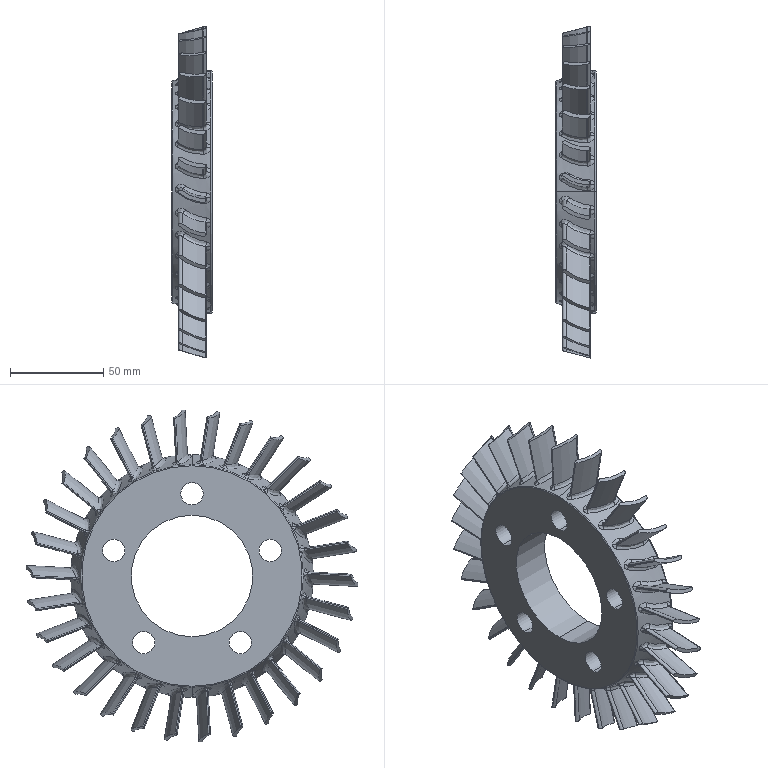Part | STEP file | Previa 01.sldasm-Part-16_Valor predeterminado | 1 solid | 636 faces | box 21.5 x 177.565 x 177.455 mm | volume 157095 mm3 | cylinder 242 | spline 210 | cone 62 | torus 50 | plane 47 | other 25 | commonest cylinder face diameters 3.2 x90 0.8 x60 42.825 x30 46.825 x30 4 x10 10 x10